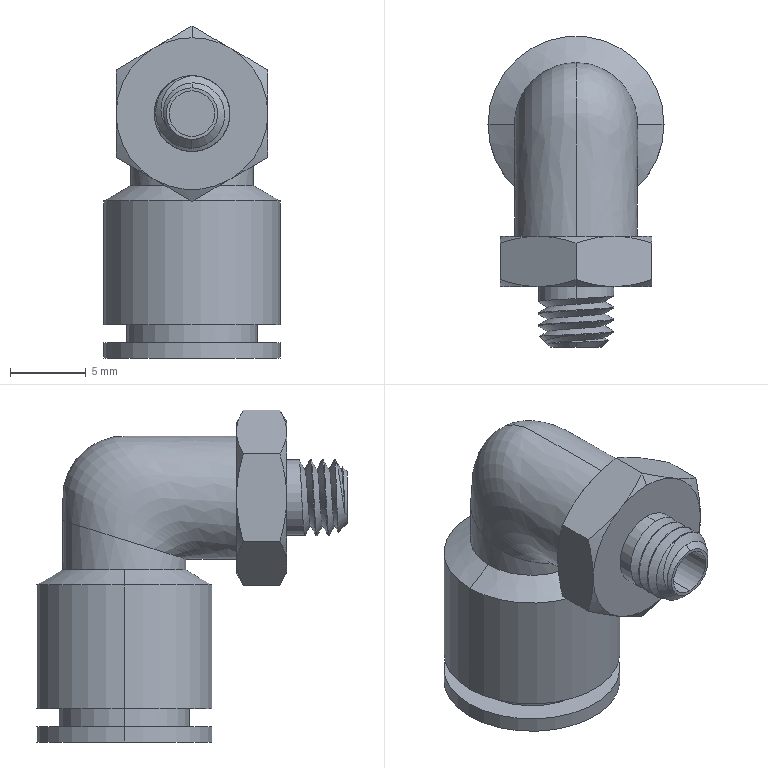Part | SolidWorks | features BaseBody 1 | 1 solid | 66 faces | box 11.6 x 20.5 x 21.874 mm | volume 1640 mm3 | cylinder 23 | plane 19 | cone 18 | spline 6 | commonest cylinder face diameters 5 x7 11.6 x4 3 x2 6 x2 8.6 x2 8.8 x2